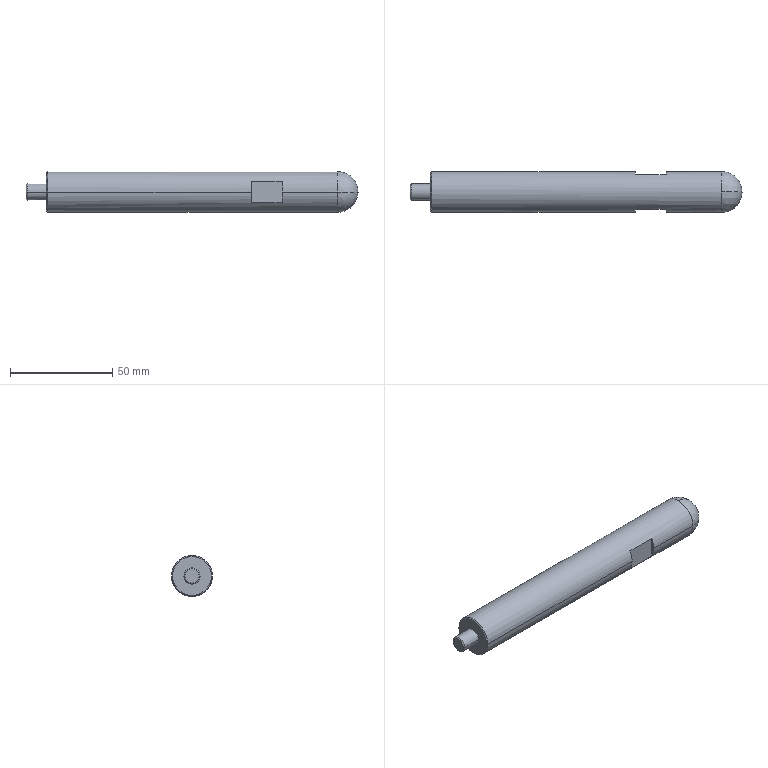Part | NX | features BREP 1 | 1 solid | 22 faces | box 162 x 20 x 20 mm | volume 46876 mm3 | plane 8 | cone 6 | cylinder 4 | sphere 4 | commonest cylinder face diameters 8 x2 20 x2
STEP:
#1=CARTESIAN_POINT('',(0.,-3.5,0.));
#2=VERTEX_POINT('',#1);
#3=CARTESIAN_POINT('',(0.,3.5,0.));
#4=VERTEX_POINT('',#3);
#5=CARTESIAN_POINT('',(0.,0.,0.));
#6=DIRECTION('',(-1.,0.,0.));
#7=DIRECTION('',(0.,-1.,0.));
#8=AXIS2_PLACEMENT_3D('',#5,#6,#7);
#9=CIRCLE('',#8,3.5);
#10=EDGE_CURVE('',#2,#4,#9,.T.);
#11=ORIENTED_EDGE('',*,*,#10,.T.);
#12=CARTESIAN_POINT('',(0.,0.,-3.5));
#13=VERTEX_POINT('',#12);
#14=CARTESIAN_POINT('',(0.,0.,0.));
#15=DIRECTION('',(-1.,0.,0.));
#16=DIRECTION('',(0.,1.,0.));
#17=AXIS2_PLACEMENT_3D('',#14,#15,#16);
#18=CIRCLE('',#17,3.5);
#19=EDGE_CURVE('',#4,#13,#18,.T.);
#20=ORIENTED_EDGE('',*,*,#19,.T.);
#21=CARTESIAN_POINT('',(0.,0.,0.));
#22=DIRECTION('',(-1.,0.,0.));
#23=DIRECTION('',(0.,1.,0.));
#24=AXIS2_PLACEMENT_3D('',#21,#22,#23);
#25=CIRCLE('',#24,3.5);
#26=EDGE_CURVE('',#13,#2,#25,.T.);
#27=ORIENTED_EDGE('',*,*,#26,.T.);
#28=EDGE_LOOP('',(#11,#20,#27));
#29=FACE_BOUND('',#28,.T.);
#30=CARTESIAN_POINT('',(0.,0.,0.));
#31=DIRECTION('',(1.,0.,0.));
#32=DIRECTION('',(0.,1.,0.));
#33=AXIS2_PLACEMENT_3D('',#30,#31,#32);
#34=PLANE('',#33);
#35=ADVANCED_FACE('',(#29),#34,.F.);
#36=CARTESIAN_POINT('',(0.5,0.,-4.));
#37=VERTEX_POINT('',#36);
#38=CARTESIAN_POINT('',(0.25,0.,-3.75));
#39=DIRECTION('',(0.7071,0.,-0.7071));
#40=VECTOR('',#39,1000.);
#41=LINE('',#38,#40);
#42=EDGE_CURVE('',#13,#37,#41,.T.);
#43=ORIENTED_EDGE('',*,*,#42,.F.);
#44=ORIENTED_EDGE('',*,*,#19,.F.);
#45=CARTESIAN_POINT('',(0.5,4.,0.));
#46=VERTEX_POINT('',#45);
#47=CARTESIAN_POINT('',(-0.000000015,3.5,0.000000086));
#48=DIRECTION('',(0.7071,0.7071,-0.000000017));
#49=VECTOR('',#48,1000.);
#50=LINE('',#47,#49);
#51=EDGE_CURVE('',#4,#46,#50,.T.);
#52=ORIENTED_EDGE('',*,*,#51,.T.);
#53=CARTESIAN_POINT('',(0.5,0.,0.));
#54=DIRECTION('',(-1.,0.,0.));
#55=DIRECTION('',(0.,1.,0.));
#56=AXIS2_PLACEMENT_3D('',#53,#54,#55);
#57=CIRCLE('',#56,4.);
#58=EDGE_CURVE('',#46,#37,#57,.T.);
#59=ORIENTED_EDGE('',*,*,#58,.T.);
#60=EDGE_LOOP('',(#43,#44,#52,#59));
#61=FACE_BOUND('',#60,.T.);
#62=CARTESIAN_POINT('',(0.25,0.,0.));
#63=DIRECTION('',(1.,0.,0.));
#64=DIRECTION('',(0.,0.,-1.));
#65=AXIS2_PLACEMENT_3D('',#62,#63,#64);
#66=CONICAL_SURFACE('',#65,3.75,0.7854);
#67=ADVANCED_FACE('',(#61),#66,.T.);
#68=CARTESIAN_POINT('',(0.5,-4.,0.));
#69=VERTEX_POINT('',#68);
#70=CARTESIAN_POINT('',(-0.000000015,-3.5,-0.000000086));
#71=DIRECTION('',(0.7071,-0.7071,0.000000017));
#72=VECTOR('',#71,1000.);
#73=LINE('',#70,#72);
#74=EDGE_CURVE('',#2,#69,#73,.T.);
#75=ORIENTED_EDGE('',*,*,#74,.T.);
#76=CARTESIAN_POINT('',(0.5,0.,0.));
#77=DIRECTION('',(-1.,0.,0.));
#78=DIRECTION('',(0.,-1.,0.));
#79=AXIS2_PLACEMENT_3D('',#76,#77,#78);
#80=CIRCLE('',#79,4.);
#81=EDGE_CURVE('',#69,#46,#80,.T.);
#82=ORIENTED_EDGE('',*,*,#81,.T.);
#83=ORIENTED_EDGE('',*,*,#51,.F.);
#84=ORIENTED_EDGE('',*,*,#10,.F.);
#85=EDGE_LOOP('',(#75,#82,#83,#84));
#86=FACE_BOUND('',#85,.T.);
#87=CARTESIAN_POINT('',(0.25,0.,0.));
#88=DIRECTION('',(1.,0.,0.));
#89=DIRECTION('',(0.,0.,-1.));
#90=AXIS2_PLACEMENT_3D('',#87,#88,#89);
#91=CONICAL_SURFACE('',#90,3.75,0.7854);
#92=ADVANCED_FACE('',(#86),#91,.T.);
#93=CARTESIAN_POINT('',(10.,-4.,0.));
#94=VERTEX_POINT('',#93);
#95=CARTESIAN_POINT('',(0.5,-4.,-0.000000074));
#96=DIRECTION('',(1.,-0.000000001,0.000000008));
#97=VECTOR('',#96,1000.);
#98=LINE('',#95,#97);
#99=EDGE_CURVE('',#69,#94,#98,.T.);
#100=ORIENTED_EDGE('',*,*,#99,.T.);
#101=CARTESIAN_POINT('',(10.,4.,0.));
#102=VERTEX_POINT('',#101);
#103=CARTESIAN_POINT('',(10.,0.,0.));
#104=DIRECTION('',(1.,0.,0.));
#105=DIRECTION('',(0.,1.,0.));
#106=AXIS2_PLACEMENT_3D('',#103,#104,#105);
#107=CIRCLE('',#106,4.);
#108=EDGE_CURVE('',#102,#94,#107,.T.);
#109=ORIENTED_EDGE('',*,*,#108,.F.);
#110=CARTESIAN_POINT('',(0.5,4.,0.000000074));
#111=DIRECTION('',(1.,0.000000001,-0.000000008));
#112=VECTOR('',#111,1000.);
#113=LINE('',#110,#112);
#114=EDGE_CURVE('',#46,#102,#113,.T.);
#115=ORIENTED_EDGE('',*,*,#114,.F.);
#116=ORIENTED_EDGE('',*,*,#81,.F.);
#117=EDGE_LOOP('',(#100,#109,#115,#116));
#118=FACE_BOUND('',#117,.T.);
#119=CARTESIAN_POINT('',(0.,0.,0.));
#120=DIRECTION('',(-1.,0.,0.));
#121=DIRECTION('',(0.,-1.,0.));
#122=AXIS2_PLACEMENT_3D('',#119,#120,#121);
#123=CYLINDRICAL_SURFACE('',#122,4.);
#124=ADVANCED_FACE('',(#118),#123,.T.);
#125=ORIENTED_EDGE('',*,*,#114,.T.);
#126=CARTESIAN_POINT('',(10.,0.,0.));
#127=DIRECTION('',(1.,0.,0.));
#128=DIRECTION('',(0.,-1.,0.));
#129=AXIS2_PLACEMENT_3D('',#126,#127,#128);
#130=CIRCLE('',#129,4.);
#131=EDGE_CURVE('',#94,#102,#130,.T.);
#132=ORIENTED_EDGE('',*,*,#131,.F.);
#133=ORIENTED_EDGE('',*,*,#99,.F.);
#134=CARTESIAN_POINT('',(0.5,0.,0.));
#135=DIRECTION('',(-1.,0.,0.));
#136=DIRECTION('',(0.,1.,0.));
#137=AXIS2_PLACEMENT_3D('',#134,#135,#136);
#138=CIRCLE('',#137,4.);
#139=EDGE_CURVE('',#37,#69,#138,.T.);
#140=ORIENTED_EDGE('',*,*,#139,.F.);
#141=ORIENTED_EDGE('',*,*,#58,.F.);
#142=EDGE_LOOP('',(#125,#132,#133,#140,#141));
#143=FACE_BOUND('',#142,.T.);
#144=CARTESIAN_POINT('',(0.,0.,0.));
#145=DIRECTION('',(-1.,0.,0.));
#146=DIRECTION('',(0.,-1.,0.));
#147=AXIS2_PLACEMENT_3D('',#144,#145,#146);
#148=CYLINDRICAL_SURFACE('',#147,4.);
#149=ADVANCED_FACE('',(#143),#148,.T.);
#150=CARTESIAN_POINT('',(10.,9.5,0.));
#151=VERTEX_POINT('',#150);
#152=CARTESIAN_POINT('',(10.,-9.5,0.));
#153=VERTEX_POINT('',#152);
#154=CARTESIAN_POINT('',(10.,0.,0.));
#155=DIRECTION('',(1.,0.,0.));
#156=DIRECTION('',(0.,1.,0.));
#157=AXIS2_PLACEMENT_3D('',#154,#155,#156);
#158=CIRCLE('',#157,9.5);
#159=EDGE_CURVE('',#151,#153,#158,.T.);
#160=ORIENTED_EDGE('',*,*,#159,.F.);
#161=CARTESIAN_POINT('',(10.,0.,-9.5));
#162=VERTEX_POINT('',#161);
#163=CARTESIAN_POINT('',(10.,0.,0.));
#164=DIRECTION('',(1.,0.,0.));
#165=DIRECTION('',(0.,-1.,0.));
#166=AXIS2_PLACEMENT_3D('',#163,#164,#165);
#167=CIRCLE('',#166,9.5);
#168=EDGE_CURVE('',#162,#151,#167,.T.);
#169=ORIENTED_EDGE('',*,*,#168,.F.);
#170=CARTESIAN_POINT('',(10.,0.,0.));
#171=DIRECTION('',(1.,0.,0.));
#172=DIRECTION('',(0.,-1.,0.));
#173=AXIS2_PLACEMENT_3D('',#170,#171,#172);
#174=CIRCLE('',#173,9.5);
#175=EDGE_CURVE('',#153,#162,#174,.T.);
#176=ORIENTED_EDGE('',*,*,#175,.F.);
#177=EDGE_LOOP('',(#160,#169,#176));
#178=FACE_BOUND('',#177,.T.);
#179=ORIENTED_EDGE('',*,*,#108,.T.);
#180=ORIENTED_EDGE('',*,*,#131,.T.);
#181=EDGE_LOOP('',(#179,#180));
#182=FACE_BOUND('',#181,.T.);
#183=CARTESIAN_POINT('',(10.,0.,0.));
#184=DIRECTION('',(-1.,0.,0.));
#185=DIRECTION('',(0.,0.,1.));
#186=AXIS2_PLACEMENT_3D('',#183,#184,#185);
#187=PLANE('',#186);
#188=ADVANCED_FACE('',(#178,#182),#187,.T.);
#189=CARTESIAN_POINT('',(10.5,0.,-10.));
#190=VERTEX_POINT('',#189);
#191=CARTESIAN_POINT('',(10.25,0.,-9.75));
#192=DIRECTION('',(0.7071,0.,-0.7071));
#193=VECTOR('',#192,1000.);
#194=LINE('',#191,#193);
#195=EDGE_CURVE('',#162,#190,#194,.T.);
#196=ORIENTED_EDGE('',*,*,#195,.F.);
#197=ORIENTED_EDGE('',*,*,#168,.T.);
#198=CARTESIAN_POINT('',(10.5,10.,0.));
#199=VERTEX_POINT('',#198);
#200=CARTESIAN_POINT('',(10.5,10.,0.));
#201=DIRECTION('',(-0.7071,-0.7071,0.));
#202=VECTOR('',#201,1000.);
#203=LINE('',#200,#202);
#204=EDGE_CURVE('',#199,#151,#203,.T.);
#205=ORIENTED_EDGE('',*,*,#204,.F.);
#206=CARTESIAN_POINT('',(10.5,0.,0.));
#207=DIRECTION('',(1.,0.,0.));
#208=DIRECTION('',(0.,-1.,0.));
#209=AXIS2_PLACEMENT_3D('',#206,#207,#208);
#210=CIRCLE('',#209,10.);
#211=EDGE_CURVE('',#190,#199,#210,.T.);
#212=ORIENTED_EDGE('',*,*,#211,.F.);
#213=EDGE_LOOP('',(#196,#197,#205,#212));
#214=FACE_BOUND('',#213,.T.);
#215=CARTESIAN_POINT('',(10.25,0.,0.));
#216=DIRECTION('',(1.,0.,0.));
#217=DIRECTION('',(0.,0.,-1.));
#218=AXIS2_PLACEMENT_3D('',#215,#216,#217);
#219=CONICAL_SURFACE('',#218,9.75,0.7854);
#220=ADVANCED_FACE('',(#214),#219,.T.);
#221=CARTESIAN_POINT('',(110.,-10.,0.));
#222=VERTEX_POINT('',#221);
#223=CARTESIAN_POINT('',(10.5,-10.,0.));
#224=VERTEX_POINT('',#223);
#225=CARTESIAN_POINT('',(110.,-10.,0.));
#226=DIRECTION('',(-1.,0.,0.));
#227=VECTOR('',#226,1000.);
#228=LINE('',#225,#227);
#229=EDGE_CURVE('',#222,#224,#228,.T.);
#230=ORIENTED_EDGE('',*,*,#229,.T.);
#231=CARTESIAN_POINT('',(10.5,0.,0.));
#232=DIRECTION('',(1.,0.,0.));
#233=DIRECTION('',(0.,-1.,0.));
#234=AXIS2_PLACEMENT_3D('',#231,#232,#233);
#235=CIRCLE('',#234,10.);
#236=EDGE_CURVE('',#224,#190,#235,.T.);
#237=ORIENTED_EDGE('',*,*,#236,.T.);
#238=ORIENTED_EDGE('',*,*,#211,.T.);
#239=CARTESIAN_POINT('',(110.,10.,0.));
#240=VERTEX_POINT('',#239);
#241=CARTESIAN_POINT('',(10.5,10.,0.));
#242=DIRECTION('',(1.,0.,0.));
#243=VECTOR('',#242,1000.);
#244=LINE('',#241,#243);
#245=EDGE_CURVE('',#199,#240,#244,.T.);
#246=ORIENTED_EDGE('',*,*,#245,.T.);
#247=CARTESIAN_POINT('',(110.,8.5,-5.268));
#248=VERTEX_POINT('',#247);
#249=CARTESIAN_POINT('',(110.,0.,0.));
#250=DIRECTION('',(-1.,0.,0.));
#251=DIRECTION('',(0.,1.,0.));
#252=AXIS2_PLACEMENT_3D('',#249,#250,#251);
#253=CIRCLE('',#252,10.);
#254=EDGE_CURVE('',#240,#248,#253,.T.);
#255=ORIENTED_EDGE('',*,*,#254,.T.);
#256=CARTESIAN_POINT('',(125.,8.5,-5.268));
#257=VERTEX_POINT('',#256);
#258=CARTESIAN_POINT('',(110.,8.5,-5.268));
#259=DIRECTION('',(1.,0.,0.));
#260=VECTOR('',#259,1000.);
#261=LINE('',#258,#260);
#262=EDGE_CURVE('',#248,#257,#261,.T.);
#263=ORIENTED_EDGE('',*,*,#262,.T.);
#264=CARTESIAN_POINT('',(125.,10.,0.));
#265=VERTEX_POINT('',#264);
#266=CARTESIAN_POINT('',(125.,0.,0.));
#267=DIRECTION('',(-1.,0.,0.));
#268=DIRECTION('',(0.,1.,0.));
#269=AXIS2_PLACEMENT_3D('',#266,#267,#268);
#270=CIRCLE('',#269,10.);
#271=EDGE_CURVE('',#265,#257,#270,.T.);
#272=ORIENTED_EDGE('',*,*,#271,.F.);
#273=CARTESIAN_POINT('',(152.,10.,0.));
#274=VERTEX_POINT('',#273);
#275=CARTESIAN_POINT('',(125.,10.,0.));
#276=DIRECTION('',(1.,0.,0.));
#277=VECTOR('',#276,1000.);
#278=LINE('',#275,#277);
#279=EDGE_CURVE('',#265,#274,#278,.T.);
#280=ORIENTED_EDGE('',*,*,#279,.T.);
#281=CARTESIAN_POINT('',(152.,5.,-8.66));
#282=VERTEX_POINT('',#281);
#283=CARTESIAN_POINT('',(152.,0.,0.));
#284=DIRECTION('',(1.,0.,0.));
#285=DIRECTION('',(0.,-1.,0.));
#286=AXIS2_PLACEMENT_3D('',#283,#284,#285);
#287=CIRCLE('',#286,10.);
#288=EDGE_CURVE('',#282,#274,#287,.T.);
#289=ORIENTED_EDGE('',*,*,#288,.F.);
#290=CARTESIAN_POINT('',(152.,-10.,0.));
#291=VERTEX_POINT('',#290);
#292=CARTESIAN_POINT('',(152.,0.,0.));
#293=DIRECTION('',(1.,0.,0.));
#294=DIRECTION('',(0.,-1.,0.));
#295=AXIS2_PLACEMENT_3D('',#292,#293,#294);
#296=CIRCLE('',#295,10.);
#297=EDGE_CURVE('',#291,#282,#296,.T.);
#298=ORIENTED_EDGE('',*,*,#297,.F.);
#299=CARTESIAN_POINT('',(125.,-10.,0.));
#300=VERTEX_POINT('',#299);
#301=CARTESIAN_POINT('',(152.,-10.,0.));
#302=DIRECTION('',(-1.,0.,0.));
#303=VECTOR('',#302,1000.);
#304=LINE('',#301,#303);
#305=EDGE_CURVE('',#291,#300,#304,.T.);
#306=ORIENTED_EDGE('',*,*,#305,.T.);
#307=CARTESIAN_POINT('',(125.,-8.5,-5.268));
#308=VERTEX_POINT('',#307);
#309=CARTESIAN_POINT('',(125.,0.,0.));
#310=DIRECTION('',(-1.,0.,0.));
#311=DIRECTION('',(0.,-0.85,-0.5268));
#312=AXIS2_PLACEMENT_3D('',#309,#310,#311);
#313=CIRCLE('',#312,10.);
#314=EDGE_CURVE('',#308,#300,#313,.T.);
#315=ORIENTED_EDGE('',*,*,#314,.F.);
#316=CARTESIAN_POINT('',(110.,-8.5,-5.268));
#317=VERTEX_POINT('',#316);
#318=CARTESIAN_POINT('',(110.,-8.5,-5.268));
#319=DIRECTION('',(1.,0.,0.));
#320=VECTOR('',#319,1000.);
#321=LINE('',#318,#320);
#322=EDGE_CURVE('',#317,#308,#321,.T.);
#323=ORIENTED_EDGE('',*,*,#322,.F.);
#324=CARTESIAN_POINT('',(110.,0.,0.));
#325=DIRECTION('',(-1.,0.,0.));
#326=DIRECTION('',(0.,-0.85,-0.5268));
#327=AXIS2_PLACEMENT_3D('',#324,#325,#326);
#328=CIRCLE('',#327,10.);
#329=EDGE_CURVE('',#317,#222,#328,.T.);
#330=ORIENTED_EDGE('',*,*,#329,.T.);
#331=EDGE_LOOP('',(#230,#237,#238,#246,#255,#263,#272,#280,#289,#298,#306,#315,#323,#330));
#332=FACE_BOUND('',#331,.T.);
#333=CARTESIAN_POINT('',(80.,0.,0.));
#334=DIRECTION('',(1.,0.,0.));
#335=DIRECTION('',(0.,1.,0.));
#336=AXIS2_PLACEMENT_3D('',#333,#334,#335);
#337=CYLINDRICAL_SURFACE('',#336,10.);
#338=ADVANCED_FACE('',(#332),#337,.T.);
#339=CARTESIAN_POINT('',(110.,8.5,5.268));
#340=VERTEX_POINT('',#339);
#341=CARTESIAN_POINT('',(110.,8.5,5.268));
#342=DIRECTION('',(0.,0.,-1.));
#343=VECTOR('',#342,1000.);
#344=LINE('',#341,#343);
#345=EDGE_CURVE('',#340,#248,#344,.T.);
#346=ORIENTED_EDGE('',*,*,#345,.T.);
#347=ORIENTED_EDGE('',*,*,#254,.F.);
#348=CARTESIAN_POINT('',(110.,0.,0.));
#349=DIRECTION('',(-1.,0.,0.));
#350=DIRECTION('',(0.,0.85,0.5268));
#351=AXIS2_PLACEMENT_3D('',#348,#349,#350);
#352=CIRCLE('',#351,10.);
#353=EDGE_CURVE('',#340,#240,#352,.T.);
#354=ORIENTED_EDGE('',*,*,#353,.F.);
#355=EDGE_LOOP('',(#346,#347,#354));
#356=FACE_BOUND('',#355,.T.);
#357=CARTESIAN_POINT('',(110.,0.,0.));
#358=DIRECTION('',(-1.,0.,0.));
#359=DIRECTION('',(0.,0.,1.));
#360=AXIS2_PLACEMENT_3D('',#357,#358,#359);
#361=PLANE('',#360);
#362=ADVANCED_FACE('',(#356),#361,.F.);
#363=ORIENTED_EDGE('',*,*,#329,.F.);
#364=CARTESIAN_POINT('',(110.,-8.5,5.268));
#365=VERTEX_POINT('',#364);
#366=CARTESIAN_POINT('',(110.,-8.5,-5.268));
#367=DIRECTION('',(0.,0.,1.));
#368=VECTOR('',#367,1000.);
#369=LINE('',#366,#368);
#370=EDGE_CURVE('',#317,#365,#369,.T.);
#371=ORIENTED_EDGE('',*,*,#370,.T.);
#372=CARTESIAN_POINT('',(110.,0.,0.));
#373=DIRECTION('',(-1.,0.,0.));
#374=DIRECTION('',(0.,-1.,0.));
#375=AXIS2_PLACEMENT_3D('',#372,#373,#374);
#376=CIRCLE('',#375,10.);
#377=EDGE_CURVE('',#222,#365,#376,.T.);
#378=ORIENTED_EDGE('',*,*,#377,.F.);
#379=EDGE_LOOP('',(#363,#371,#378));
#380=FACE_BOUND('',#379,.T.);
#381=CARTESIAN_POINT('',(110.,0.,0.));
#382=DIRECTION('',(-1.,0.,0.));
#383=DIRECTION('',(0.,0.,1.));
#384=AXIS2_PLACEMENT_3D('',#381,#382,#383);
#385=PLANE('',#384);
#386=ADVANCED_FACE('',(#380),#385,.F.);
#387=ORIENTED_EDGE('',*,*,#245,.F.);
#388=CARTESIAN_POINT('',(10.5,0.,0.));
#389=DIRECTION('',(1.,0.,0.));
#390=DIRECTION('',(0.,1.,0.));
#391=AXIS2_PLACEMENT_3D('',#388,#389,#390);
#392=CIRCLE('',#391,10.);
#393=EDGE_CURVE('',#199,#224,#392,.T.);
#394=ORIENTED_EDGE('',*,*,#393,.T.);
#395=ORIENTED_EDGE('',*,*,#229,.F.);
#396=ORIENTED_EDGE('',*,*,#377,.T.);
#397=CARTESIAN_POINT('',(125.,-8.5,5.268));
#398=VERTEX_POINT('',#397);
#399=CARTESIAN_POINT('',(110.,-8.5,5.268));
#400=DIRECTION('',(1.,0.,0.));
#401=VECTOR('',#400,1000.);
#402=LINE('',#399,#401);
#403=EDGE_CURVE('',#365,#398,#402,.T.);
#404=ORIENTED_EDGE('',*,*,#403,.T.);
#405=CARTESIAN_POINT('',(125.,0.,0.));
#406=DIRECTION('',(-1.,0.,0.));
#407=DIRECTION('',(0.,-1.,0.));
#408=AXIS2_PLACEMENT_3D('',#405,#406,#407);
#409=CIRCLE('',#408,10.);
#410=EDGE_CURVE('',#300,#398,#409,.T.);
#411=ORIENTED_EDGE('',*,*,#410,.F.);
#412=ORIENTED_EDGE('',*,*,#305,.F.);
#413=CARTESIAN_POINT('',(152.,0.,10.));
#414=VERTEX_POINT('',#413);
#415=CARTESIAN_POINT('',(152.,0.,0.));
#416=DIRECTION('',(1.,0.,0.));
#417=DIRECTION('',(0.,1.,0.));
#418=AXIS2_PLACEMENT_3D('',#415,#416,#417);
#419=CIRCLE('',#418,10.);
#420=EDGE_CURVE('',#414,#291,#419,.T.);
#421=ORIENTED_EDGE('',*,*,#420,.F.);
#422=CARTESIAN_POINT('',(152.,0.,0.));
#423=DIRECTION('',(1.,0.,0.));
#424=DIRECTION('',(0.,1.,0.));
#425=AXIS2_PLACEMENT_3D('',#422,#423,#424);
#426=CIRCLE('',#425,10.);
#427=EDGE_CURVE('',#274,#414,#426,.T.);
#428=ORIENTED_EDGE('',*,*,#427,.F.);
#429=ORIENTED_EDGE('',*,*,#279,.F.);
#430=CARTESIAN_POINT('',(125.,8.5,5.268));
#431=VERTEX_POINT('',#430);
#432=CARTESIAN_POINT('',(125.,0.,0.));
#433=DIRECTION('',(-1.,0.,0.));
#434=DIRECTION('',(0.,0.85,0.5268));
#435=AXIS2_PLACEMENT_3D('',#432,#433,#434);
#436=CIRCLE('',#435,10.);
#437=EDGE_CURVE('',#431,#265,#436,.T.);
#438=ORIENTED_EDGE('',*,*,#437,.F.);
#439=CARTESIAN_POINT('',(110.,8.5,5.268));
#440=DIRECTION('',(1.,0.,0.));
#441=VECTOR('',#440,1000.);
#442=LINE('',#439,#441);
#443=EDGE_CURVE('',#340,#431,#442,.T.);
#444=ORIENTED_EDGE('',*,*,#443,.F.);
#445=ORIENTED_EDGE('',*,*,#353,.T.);
#446=EDGE_LOOP('',(#387,#394,#395,#396,#404,#411,#412,#421,#428,#429,#438,#444,#445));
#447=FACE_BOUND('',#446,.T.);
#448=CARTESIAN_POINT('',(80.,0.,0.));
#449=DIRECTION('',(1.,0.,0.));
#450=DIRECTION('',(0.,1.,0.));
#451=AXIS2_PLACEMENT_3D('',#448,#449,#450);
#452=CYLINDRICAL_SURFACE('',#451,10.);
#453=ADVANCED_FACE('',(#447),#452,.T.);
#454=CARTESIAN_POINT('',(125.,8.5,5.268));
#455=DIRECTION('',(0.,0.,-1.));
#456=VECTOR('',#455,1000.);
#457=LINE('',#454,#456);
#458=EDGE_CURVE('',#431,#257,#457,.T.);
#459=ORIENTED_EDGE('',*,*,#458,.T.);
#460=ORIENTED_EDGE('',*,*,#262,.F.);
#461=ORIENTED_EDGE('',*,*,#345,.F.);
#462=ORIENTED_EDGE('',*,*,#443,.T.);
#463=EDGE_LOOP('',(#459,#460,#461,#462));
#464=FACE_BOUND('',#463,.T.);
#465=CARTESIAN_POINT('',(110.,8.5,-12.5));
#466=DIRECTION('',(0.,-1.,0.));
#467=DIRECTION('',(0.,0.,-1.));
#468=AXIS2_PLACEMENT_3D('',#465,#466,#467);
#469=PLANE('',#468);
#470=ADVANCED_FACE('',(#464),#469,.F.);
#471=ORIENTED_EDGE('',*,*,#271,.T.);
#472=ORIENTED_EDGE('',*,*,#458,.F.);
#473=ORIENTED_EDGE('',*,*,#437,.T.);
#474=EDGE_LOOP('',(#471,#472,#473));
#475=FACE_BOUND('',#474,.T.);
#476=CARTESIAN_POINT('',(125.,0.,0.));
#477=DIRECTION('',(-1.,0.,0.));
#478=DIRECTION('',(0.,0.,1.));
#479=AXIS2_PLACEMENT_3D('',#476,#477,#478);
#480=PLANE('',#479);
#481=ADVANCED_FACE('',(#475),#480,.T.);
#482=CARTESIAN_POINT('',(125.,-8.5,-5.268));
#483=DIRECTION('',(0.,0.,1.));
#484=VECTOR('',#483,1000.);
#485=LINE('',#482,#484);
#486=EDGE_CURVE('',#308,#398,#485,.T.);
#487=ORIENTED_EDGE('',*,*,#486,.F.);
#488=ORIENTED_EDGE('',*,*,#314,.T.);
#489=ORIENTED_EDGE('',*,*,#410,.T.);
#490=EDGE_LOOP('',(#487,#488,#489));
#491=FACE_BOUND('',#490,.T.);
#492=CARTESIAN_POINT('',(125.,0.,0.));
#493=DIRECTION('',(-1.,0.,0.));
#494=DIRECTION('',(0.,0.,1.));
#495=AXIS2_PLACEMENT_3D('',#492,#493,#494);
#496=PLANE('',#495);
#497=ADVANCED_FACE('',(#491),#496,.T.);
#498=ORIENTED_EDGE('',*,*,#370,.F.);
#499=ORIENTED_EDGE('',*,*,#322,.T.);
#500=ORIENTED_EDGE('',*,*,#486,.T.);
#501=ORIENTED_EDGE('',*,*,#403,.F.);
#502=EDGE_LOOP('',(#498,#499,#500,#501));
#503=FACE_BOUND('',#502,.T.);
#504=CARTESIAN_POINT('',(110.,-8.5,12.5));
#505=DIRECTION('',(0.,1.,0.));
#506=DIRECTION('',(1.,0.,0.));
#507=AXIS2_PLACEMENT_3D('',#504,#505,#506);
#508=PLANE('',#507);
#509=ADVANCED_FACE('',(#503),#508,.F.);
#510=CARTESIAN_POINT('',(162.,0.,0.));
#511=VERTEX_POINT('',#510);
#512=CARTESIAN_POINT('',(152.,0.,0.));
#513=DIRECTION('',(0.,1.,0.));
#514=DIRECTION('',(0.,0.,1.));
#515=AXIS2_PLACEMENT_3D('',#512,#513,#514);
#516=CIRCLE('',#515,10.);
#517=EDGE_CURVE('',#414,#511,#516,.T.);
#518=ORIENTED_EDGE('',*,*,#517,.F.);
#519=ORIENTED_EDGE('',*,*,#420,.T.);
#520=CARTESIAN_POINT('',(152.,0.,0.));
#521=DIRECTION('',(0.,0.,-1.));
#522=DIRECTION('',(1.,0.,0.));
#523=AXIS2_PLACEMENT_3D('',#520,#521,#522);
#524=CIRCLE('',#523,10.);
#525=EDGE_CURVE('',#511,#291,#524,.T.);
#526=ORIENTED_EDGE('',*,*,#525,.F.);
#527=EDGE_LOOP('',(#518,#519,#526));
#528=FACE_BOUND('',#527,.T.);
#529=CARTESIAN_POINT('',(152.,0.,0.));
#530=DIRECTION('',(0.,-1.,0.));
#531=DIRECTION('',(0.,0.,1.));
#532=AXIS2_PLACEMENT_3D('',#529,#530,#531);
#533=SPHERICAL_SURFACE('',#532,10.);
#534=ADVANCED_FACE('',(#528),#533,.T.);
#535=CARTESIAN_POINT('',(152.,0.,0.));
#536=DIRECTION('',(0.,-0.866,-0.5));
#537=DIRECTION('',(0.,0.5,-0.866));
#538=AXIS2_PLACEMENT_3D('',#535,#536,#537);
#539=CIRCLE('',#538,10.);
#540=EDGE_CURVE('',#282,#511,#539,.T.);
#541=ORIENTED_EDGE('',*,*,#540,.F.);
#542=ORIENTED_EDGE('',*,*,#288,.T.);
#543=CARTESIAN_POINT('',(152.,0.,0.));
#544=DIRECTION('',(0.,0.,-1.));
#545=DIRECTION('',(1.,0.,0.));
#546=AXIS2_PLACEMENT_3D('',#543,#544,#545);
#547=CIRCLE('',#546,10.);
#548=EDGE_CURVE('',#274,#511,#547,.T.);
#549=ORIENTED_EDGE('',*,*,#548,.T.);
#550=EDGE_LOOP('',(#541,#542,#549));
#551=FACE_BOUND('',#550,.T.);
#552=CARTESIAN_POINT('',(152.,0.,0.));
#553=DIRECTION('',(0.,0.866,0.5));
#554=DIRECTION('',(0.,0.5,-0.866));
#555=AXIS2_PLACEMENT_3D('',#552,#553,#554);
#556=SPHERICAL_SURFACE('',#555,10.);
#557=ADVANCED_FACE('',(#551),#556,.T.);
#558=ORIENTED_EDGE('',*,*,#204,.T.);
#559=ORIENTED_EDGE('',*,*,#159,.T.);
#560=CARTESIAN_POINT('',(10.5,-10.,0.));
#561=DIRECTION('',(-0.7071,0.7071,0.));
#562=VECTOR('',#561,1000.);
#563=LINE('',#560,#562);
#564=EDGE_CURVE('',#224,#153,#563,.T.);
#565=ORIENTED_EDGE('',*,*,#564,.F.);
#566=ORIENTED_EDGE('',*,*,#393,.F.);
#567=EDGE_LOOP('',(#558,#559,#565,#566));
#568=FACE_BOUND('',#567,.T.);
#569=CARTESIAN_POINT('',(10.25,0.,0.));
#570=DIRECTION('',(1.,0.,0.));
#571=DIRECTION('',(0.,0.,-1.));
#572=AXIS2_PLACEMENT_3D('',#569,#570,#571);
#573=CONICAL_SURFACE('',#572,9.75,0.7854);
#574=ADVANCED_FACE('',(#568),#573,.T.);
#575=ORIENTED_EDGE('',*,*,#297,.T.);
#576=ORIENTED_EDGE('',*,*,#540,.T.);
#577=ORIENTED_EDGE('',*,*,#525,.T.);
#578=EDGE_LOOP('',(#575,#576,#577));
#579=FACE_BOUND('',#578,.T.);
#580=CARTESIAN_POINT('',(152.,0.,0.));
#581=DIRECTION('',(0.,0.866,0.5));
#582=DIRECTION('',(0.,0.5,-0.866));
#583=AXIS2_PLACEMENT_3D('',#580,#581,#582);
#584=SPHERICAL_SURFACE('',#583,10.);
#585=ADVANCED_FACE('',(#579),#584,.T.);
#586=ORIENTED_EDGE('',*,*,#427,.T.);
#587=ORIENTED_EDGE('',*,*,#517,.T.);
#588=ORIENTED_EDGE('',*,*,#548,.F.);
#589=EDGE_LOOP('',(#586,#587,#588));
#590=FACE_BOUND('',#589,.T.);
#591=CARTESIAN_POINT('',(152.,0.,0.));
#592=DIRECTION('',(0.,-1.,0.));
#593=DIRECTION('',(0.,0.,1.));
#594=AXIS2_PLACEMENT_3D('',#591,#592,#593);
#595=SPHERICAL_SURFACE('',#594,10.);
#596=ADVANCED_FACE('',(#590),#595,.T.);
#597=ORIENTED_EDGE('',*,*,#175,.T.);
#598=ORIENTED_EDGE('',*,*,#195,.T.);
#599=ORIENTED_EDGE('',*,*,#236,.F.);
#600=ORIENTED_EDGE('',*,*,#564,.T.);
#601=EDGE_LOOP('',(#597,#598,#599,#600));
#602=FACE_BOUND('',#601,.T.);
#603=CARTESIAN_POINT('',(10.25,0.,0.));
#604=DIRECTION('',(1.,0.,0.));
#605=DIRECTION('',(0.,0.,-1.));
#606=AXIS2_PLACEMENT_3D('',#603,#604,#605);
#607=CONICAL_SURFACE('',#606,9.75,0.7854);
#608=ADVANCED_FACE('',(#602),#607,.T.);
#609=ORIENTED_EDGE('',*,*,#26,.F.);
#610=ORIENTED_EDGE('',*,*,#42,.T.);
#611=ORIENTED_EDGE('',*,*,#139,.T.);
#612=ORIENTED_EDGE('',*,*,#74,.F.);
#613=EDGE_LOOP('',(#609,#610,#611,#612));
#614=FACE_BOUND('',#613,.T.);
#615=CARTESIAN_POINT('',(0.25,0.,0.));
#616=DIRECTION('',(1.,0.,0.));
#617=DIRECTION('',(0.,0.,-1.));
#618=AXIS2_PLACEMENT_3D('',#615,#616,#617);
#619=CONICAL_SURFACE('',#618,3.75,0.7854);
#620=ADVANCED_FACE('',(#614),#619,.T.);
#621=CLOSED_SHELL('',(#35,#67,#92,#124,#149,#188,#220,#338,#362,#386,#453,#470,#481,#497,#509,#534,#557,#574,#585,#596,#608,#620));
#622=MANIFOLD_SOLID_BREP('',#621);
#623=(LENGTH_UNIT()NAMED_UNIT(*)SI_UNIT(.MILLI.,.METRE.));
#624=UNCERTAINTY_MEASURE_WITH_UNIT(LENGTH_MEASURE(0.00001),#623,'','');
#625=(NAMED_UNIT(*)PLANE_ANGLE_UNIT()SI_UNIT($,.RADIAN.));
#626=(NAMED_UNIT(*)SI_UNIT($,.STERADIAN.)SOLID_ANGLE_UNIT());
#627=(GEOMETRIC_REPRESENTATION_CONTEXT(3)GLOBAL_UNCERTAINTY_ASSIGNED_CONTEXT((#624))GLOBAL_UNIT_ASSIGNED_CONTEXT((#623,#625,#626))REPRESENTATION_CONTEXT('',''));
#628=ADVANCED_BREP_SHAPE_REPRESENTATION('',(#622),#627);